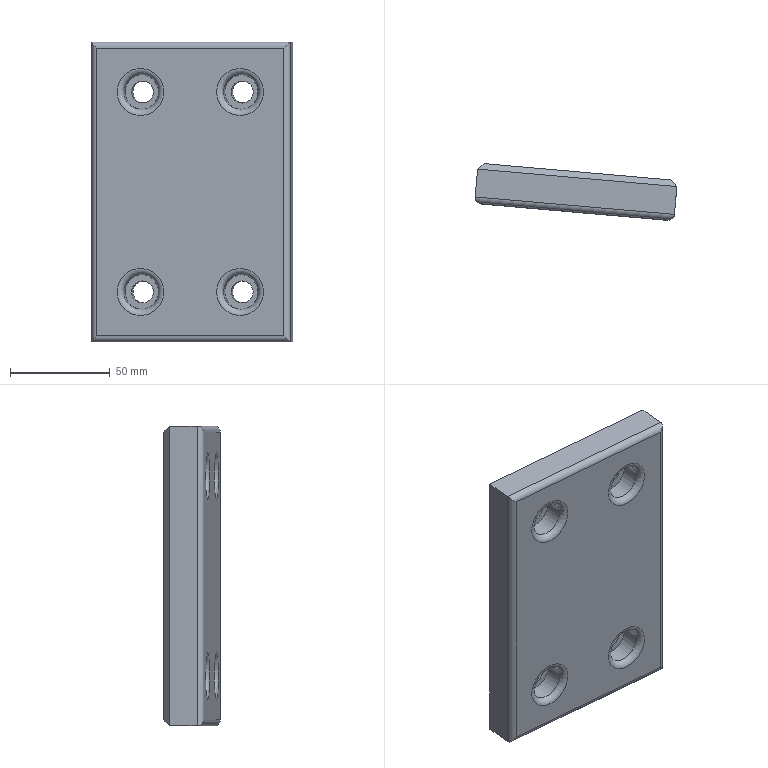Part | NX | features MAIN_BODY 2 | 1 solid | 30 faces | box 100.851 x 28.128 x 150 mm | volume 281787 mm3 | plane 14 | cylinder 12 | torus 4 | commonest cylinder face diameters 6 x4 11 x4 17.5 x4
STEP:
#1=CARTESIAN_POINT('',(223.712,-345.814,-117.));
#2=VERTEX_POINT('',#1);
#3=CARTESIAN_POINT('',(223.712,-345.814,27.));
#4=VERTEX_POINT('',#3);
#5=CARTESIAN_POINT('',(223.712,-345.814,30.));
#6=DIRECTION('',(0.,0.,-1.));
#7=VECTOR('',#6,1000.);
#8=LINE('',#5,#7);
#9=EDGE_CURVE('',#2,#4,#8,.F.);
#10=ORIENTED_EDGE('',*,*,#9,.F.);
#11=CARTESIAN_POINT('',(317.354,-354.006,-117.));
#12=VERTEX_POINT('',#11);
#13=CARTESIAN_POINT('',(190.837,-342.938,-117.));
#14=DIRECTION('',(0.9962,-0.08716,0.));
#15=VECTOR('',#14,1000.);
#16=LINE('',#13,#15);
#17=EDGE_CURVE('',#12,#2,#16,.F.);
#18=ORIENTED_EDGE('',*,*,#17,.F.);
#19=CARTESIAN_POINT('',(317.354,-354.006,27.));
#20=VERTEX_POINT('',#19);
#21=CARTESIAN_POINT('',(317.354,-354.006,-170.));
#22=DIRECTION('',(0.,0.,1.));
#23=VECTOR('',#22,1000.);
#24=LINE('',#21,#23);
#25=EDGE_CURVE('',#20,#12,#24,.F.);
#26=ORIENTED_EDGE('',*,*,#25,.F.);
#27=CARTESIAN_POINT('',(340.266,-356.011,27.));
#28=DIRECTION('',(-0.9962,0.08716,0.));
#29=VECTOR('',#28,1000.);
#30=LINE('',#27,#29);
#31=EDGE_CURVE('',#4,#20,#30,.F.);
#32=ORIENTED_EDGE('',*,*,#31,.F.);
#33=EDGE_LOOP('',(#10,#18,#26,#32));
#34=FACE_BOUND('',#33,.T.);
#35=CARTESIAN_POINT('',(245.628,-347.731,-6.75));
#36=VERTEX_POINT('',#35);
#37=CARTESIAN_POINT('',(245.628,-347.731,5.));
#38=DIRECTION('',(-0.08716,-0.9962,0.));
#39=DIRECTION('',(0.,0.,-1.));
#40=AXIS2_PLACEMENT_3D('',#37,#38,#39);
#41=CIRCLE('',#40,11.75);
#42=EDGE_CURVE('',#36,#36,#41,.T.);
#43=ORIENTED_EDGE('',*,*,#42,.F.);
#44=EDGE_LOOP('',(#43));
#45=FACE_BOUND('',#44,.T.);
#46=CARTESIAN_POINT('',(295.438,-352.089,-6.75));
#47=VERTEX_POINT('',#46);
#48=CARTESIAN_POINT('',(295.438,-352.089,5.));
#49=DIRECTION('',(-0.08716,-0.9962,0.));
#50=DIRECTION('',(0.,0.,-1.));
#51=AXIS2_PLACEMENT_3D('',#48,#49,#50);
#52=CIRCLE('',#51,11.75);
#53=EDGE_CURVE('',#47,#47,#52,.T.);
#54=ORIENTED_EDGE('',*,*,#53,.F.);
#55=EDGE_LOOP('',(#54));
#56=FACE_BOUND('',#55,.T.);
#57=CARTESIAN_POINT('',(295.438,-352.089,-106.75));
#58=VERTEX_POINT('',#57);
#59=CARTESIAN_POINT('',(295.438,-352.089,-95.));
#60=DIRECTION('',(-0.08716,-0.9962,0.));
#61=DIRECTION('',(0.,0.,-1.));
#62=AXIS2_PLACEMENT_3D('',#59,#60,#61);
#63=CIRCLE('',#62,11.75);
#64=EDGE_CURVE('',#58,#58,#63,.T.);
#65=ORIENTED_EDGE('',*,*,#64,.F.);
#66=EDGE_LOOP('',(#65));
#67=FACE_BOUND('',#66,.T.);
#68=CARTESIAN_POINT('',(245.628,-347.731,-106.75));
#69=VERTEX_POINT('',#68);
#70=CARTESIAN_POINT('',(245.628,-347.731,-95.));
#71=DIRECTION('',(-0.08716,-0.9962,0.));
#72=DIRECTION('',(0.,0.,-1.));
#73=AXIS2_PLACEMENT_3D('',#70,#71,#72);
#74=CIRCLE('',#73,11.75);
#75=EDGE_CURVE('',#69,#69,#74,.T.);
#76=ORIENTED_EDGE('',*,*,#75,.F.);
#77=EDGE_LOOP('',(#76));
#78=FACE_BOUND('',#77,.T.);
#79=CARTESIAN_POINT('',(190.837,-342.938,-170.));
#80=DIRECTION('',(0.08716,0.9962,0.));
#81=DIRECTION('',(0.,0.,-1.));
#82=AXIS2_PLACEMENT_3D('',#79,#80,#81);
#83=PLANE('',#82);
#84=ADVANCED_FACE('',(#34,#45,#56,#67,#78),#83,.F.);
#85=CARTESIAN_POINT('',(291.702,-331.686,-95.));
#86=VERTEX_POINT('',#85);
#87=CARTESIAN_POINT('',(297.181,-332.165,-95.));
#88=DIRECTION('',(0.08716,0.9962,0.));
#89=DIRECTION('',(-0.9962,0.08716,0.));
#90=AXIS2_PLACEMENT_3D('',#87,#88,#89);
#91=CIRCLE('',#90,5.5);
#92=EDGE_CURVE('',#86,#86,#91,.T.);
#93=ORIENTED_EDGE('',*,*,#92,.T.);
#94=EDGE_LOOP('',(#93));
#95=FACE_BOUND('',#94,.T.);
#96=CARTESIAN_POINT('',(296.484,-340.135,-89.5));
#97=VERTEX_POINT('',#96);
#98=CARTESIAN_POINT('',(296.484,-340.135,-95.));
#99=DIRECTION('',(0.08716,0.9962,0.));
#100=DIRECTION('',(0.,0.,1.));
#101=AXIS2_PLACEMENT_3D('',#98,#99,#100);
#102=CIRCLE('',#101,5.5);
#103=EDGE_CURVE('',#97,#97,#102,.T.);
#104=ORIENTED_EDGE('',*,*,#103,.F.);
#105=EDGE_LOOP('',(#104));
#106=FACE_BOUND('',#105,.T.);
#107=CARTESIAN_POINT('',(295.438,-352.089,-95.));
#108=DIRECTION('',(0.08716,0.9962,0.));
#109=DIRECTION('',(0.,0.,-1.));
#110=AXIS2_PLACEMENT_3D('',#107,#108,#109);
#111=CYLINDRICAL_SURFACE('',#110,5.5);
#112=ADVANCED_FACE('',(#95,#106),#111,.F.);
#113=CARTESIAN_POINT('',(252.85,-328.287,5.));
#114=VERTEX_POINT('',#113);
#115=CARTESIAN_POINT('',(247.371,-327.807,5.));
#116=DIRECTION('',(0.08716,0.9962,0.));
#117=DIRECTION('',(0.9962,-0.08716,0.));
#118=AXIS2_PLACEMENT_3D('',#115,#116,#117);
#119=CIRCLE('',#118,5.5);
#120=EDGE_CURVE('',#114,#114,#119,.T.);
#121=ORIENTED_EDGE('',*,*,#120,.T.);
#122=EDGE_LOOP('',(#121));
#123=FACE_BOUND('',#122,.T.);
#124=CARTESIAN_POINT('',(246.674,-335.777,10.5));
#125=VERTEX_POINT('',#124);
#126=CARTESIAN_POINT('',(246.674,-335.777,5.));
#127=DIRECTION('',(0.08716,0.9962,0.));
#128=DIRECTION('',(0.,0.,1.));
#129=AXIS2_PLACEMENT_3D('',#126,#127,#128);
#130=CIRCLE('',#129,5.5);
#131=EDGE_CURVE('',#125,#125,#130,.T.);
#132=ORIENTED_EDGE('',*,*,#131,.F.);
#133=EDGE_LOOP('',(#132));
#134=FACE_BOUND('',#133,.T.);
#135=CARTESIAN_POINT('',(245.628,-347.731,5.));
#136=DIRECTION('',(0.08716,0.9962,0.));
#137=DIRECTION('',(0.,0.,-1.));
#138=AXIS2_PLACEMENT_3D('',#135,#136,#137);
#139=CYLINDRICAL_SURFACE('',#138,5.5);
#140=ADVANCED_FACE('',(#123,#134),#139,.F.);
#141=CARTESIAN_POINT('',(319.097,-334.082,-117.));
#142=VERTEX_POINT('',#141);
#143=CARTESIAN_POINT('',(319.097,-334.082,27.));
#144=VERTEX_POINT('',#143);
#145=CARTESIAN_POINT('',(319.097,-334.082,-170.));
#146=DIRECTION('',(0.,0.,1.));
#147=VECTOR('',#146,1000.);
#148=LINE('',#145,#147);
#149=EDGE_CURVE('',#142,#144,#148,.T.);
#150=ORIENTED_EDGE('',*,*,#149,.F.);
#151=CARTESIAN_POINT('',(225.455,-325.89,-117.));
#152=VERTEX_POINT('',#151);
#153=CARTESIAN_POINT('',(192.58,-323.014,-117.));
#154=DIRECTION('',(0.9962,-0.08716,0.));
#155=VECTOR('',#154,1000.);
#156=LINE('',#153,#155);
#157=EDGE_CURVE('',#152,#142,#156,.T.);
#158=ORIENTED_EDGE('',*,*,#157,.F.);
#159=CARTESIAN_POINT('',(225.455,-325.89,27.));
#160=VERTEX_POINT('',#159);
#161=CARTESIAN_POINT('',(225.455,-325.89,-170.));
#162=DIRECTION('',(0.,0.,-1.));
#163=VECTOR('',#162,1000.);
#164=LINE('',#161,#163);
#165=EDGE_CURVE('',#160,#152,#164,.T.);
#166=ORIENTED_EDGE('',*,*,#165,.F.);
#167=CARTESIAN_POINT('',(192.58,-323.014,27.));
#168=DIRECTION('',(-0.9962,0.08716,0.));
#169=VECTOR('',#168,1000.);
#170=LINE('',#167,#169);
#171=EDGE_CURVE('',#144,#160,#170,.T.);
#172=ORIENTED_EDGE('',*,*,#171,.F.);
#173=EDGE_LOOP('',(#150,#158,#166,#172));
#174=FACE_BOUND('',#173,.T.);
#175=CARTESIAN_POINT('',(252.85,-328.287,-95.));
#176=VERTEX_POINT('',#175);
#177=CARTESIAN_POINT('',(247.371,-327.807,-95.));
#178=DIRECTION('',(-0.08716,-0.9962,0.));
#179=DIRECTION('',(0.9962,-0.08716,0.));
#180=AXIS2_PLACEMENT_3D('',#177,#178,#179);
#181=CIRCLE('',#180,5.5);
#182=EDGE_CURVE('',#176,#176,#181,.T.);
#183=ORIENTED_EDGE('',*,*,#182,.T.);
#184=EDGE_LOOP('',(#183));
#185=FACE_BOUND('',#184,.T.);
#186=ORIENTED_EDGE('',*,*,#92,.F.);
#187=EDGE_LOOP('',(#186));
#188=FACE_BOUND('',#187,.T.);
#189=CARTESIAN_POINT('',(291.702,-331.686,5.));
#190=VERTEX_POINT('',#189);
#191=CARTESIAN_POINT('',(297.181,-332.165,5.));
#192=DIRECTION('',(-0.08716,-0.9962,0.));
#193=DIRECTION('',(-0.9962,0.08716,0.));
#194=AXIS2_PLACEMENT_3D('',#191,#192,#193);
#195=CIRCLE('',#194,5.5);
#196=EDGE_CURVE('',#190,#190,#195,.T.);
#197=ORIENTED_EDGE('',*,*,#196,.T.);
#198=EDGE_LOOP('',(#197));
#199=FACE_BOUND('',#198,.T.);
#200=ORIENTED_EDGE('',*,*,#120,.F.);
#201=EDGE_LOOP('',(#200));
#202=FACE_BOUND('',#201,.T.);
#203=CARTESIAN_POINT('',(192.58,-323.014,-170.));
#204=DIRECTION('',(0.08716,0.9962,0.));
#205=DIRECTION('',(0.,0.,-1.));
#206=AXIS2_PLACEMENT_3D('',#203,#204,#205);
#207=PLANE('',#206);
#208=ADVANCED_FACE('',(#174,#185,#188,#199,#202),#207,.T.);
#209=CARTESIAN_POINT('',(220.985,-342.564,-120.));
#210=VERTEX_POINT('',#209);
#211=CARTESIAN_POINT('',(222.205,-328.617,-120.));
#212=VERTEX_POINT('',#211);
#213=CARTESIAN_POINT('',(220.723,-345.552,-120.));
#214=DIRECTION('',(0.08716,0.9962,0.));
#215=VECTOR('',#214,1000.);
#216=LINE('',#213,#215);
#217=EDGE_CURVE('',#210,#212,#216,.T.);
#218=ORIENTED_EDGE('',*,*,#217,.F.);
#219=CARTESIAN_POINT('',(220.985,-342.564,30.));
#220=VERTEX_POINT('',#219);
#221=CARTESIAN_POINT('',(220.985,-342.564,-170.));
#222=DIRECTION('',(0.,0.,-1.));
#223=VECTOR('',#222,1000.);
#224=LINE('',#221,#223);
#225=EDGE_CURVE('',#220,#210,#224,.T.);
#226=ORIENTED_EDGE('',*,*,#225,.F.);
#227=CARTESIAN_POINT('',(222.205,-328.617,30.));
#228=VERTEX_POINT('',#227);
#229=CARTESIAN_POINT('',(220.723,-345.552,30.));
#230=DIRECTION('',(0.08716,0.9962,0.));
#231=VECTOR('',#230,1000.);
#232=LINE('',#229,#231);
#233=EDGE_CURVE('',#220,#228,#232,.T.);
#234=ORIENTED_EDGE('',*,*,#233,.T.);
#235=CARTESIAN_POINT('',(222.205,-328.617,30.));
#236=DIRECTION('',(0.,0.,1.));
#237=VECTOR('',#236,1000.);
#238=LINE('',#235,#237);
#239=EDGE_CURVE('',#212,#228,#238,.T.);
#240=ORIENTED_EDGE('',*,*,#239,.F.);
#241=EDGE_LOOP('',(#218,#226,#234,#240));
#242=FACE_BOUND('',#241,.T.);
#243=CARTESIAN_POINT('',(220.723,-345.552,30.));
#244=DIRECTION('',(-0.9962,0.08716,0.));
#245=DIRECTION('',(0.,0.,1.));
#246=AXIS2_PLACEMENT_3D('',#243,#244,#245);
#247=PLANE('',#246);
#248=ADVANCED_FACE('',(#242),#247,.T.);
#249=CARTESIAN_POINT('',(320.604,-351.279,-120.));
#250=VERTEX_POINT('',#249);
#251=CARTESIAN_POINT('',(321.824,-337.332,-120.));
#252=VERTEX_POINT('',#251);
#253=CARTESIAN_POINT('',(320.343,-354.268,-120.));
#254=DIRECTION('',(0.08716,0.9962,0.));
#255=VECTOR('',#254,1000.);
#256=LINE('',#253,#255);
#257=EDGE_CURVE('',#250,#252,#256,.T.);
#258=ORIENTED_EDGE('',*,*,#257,.F.);
#259=CARTESIAN_POINT('',(340.528,-353.022,-120.));
#260=DIRECTION('',(0.9962,-0.08716,0.));
#261=VECTOR('',#260,1000.);
#262=LINE('',#259,#261);
#263=EDGE_CURVE('',#210,#250,#262,.T.);
#264=ORIENTED_EDGE('',*,*,#263,.F.);
#265=ORIENTED_EDGE('',*,*,#217,.T.);
#266=CARTESIAN_POINT('',(192.319,-326.002,-120.));
#267=DIRECTION('',(-0.9962,0.08716,0.));
#268=VECTOR('',#267,1000.);
#269=LINE('',#266,#268);
#270=EDGE_CURVE('',#252,#212,#269,.T.);
#271=ORIENTED_EDGE('',*,*,#270,.F.);
#272=EDGE_LOOP('',(#258,#264,#265,#271));
#273=FACE_BOUND('',#272,.T.);
#274=CARTESIAN_POINT('',(190.837,-342.938,-120.));
#275=DIRECTION('',(0.,0.,-1.));
#276=DIRECTION('',(-0.9962,0.08716,0.));
#277=AXIS2_PLACEMENT_3D('',#274,#275,#276);
#278=PLANE('',#277);
#279=ADVANCED_FACE('',(#273),#278,.T.);
#280=CARTESIAN_POINT('',(320.604,-351.279,30.));
#281=VERTEX_POINT('',#280);
#282=CARTESIAN_POINT('',(321.824,-337.332,30.));
#283=VERTEX_POINT('',#282);
#284=CARTESIAN_POINT('',(320.343,-354.268,30.));
#285=DIRECTION('',(0.08716,0.9962,0.));
#286=VECTOR('',#285,1000.);
#287=LINE('',#284,#286);
#288=EDGE_CURVE('',#281,#283,#287,.T.);
#289=ORIENTED_EDGE('',*,*,#288,.F.);
#290=CARTESIAN_POINT('',(320.604,-351.279,30.));
#291=DIRECTION('',(0.,0.,1.));
#292=VECTOR('',#291,1000.);
#293=LINE('',#290,#292);
#294=EDGE_CURVE('',#250,#281,#293,.T.);
#295=ORIENTED_EDGE('',*,*,#294,.F.);
#296=ORIENTED_EDGE('',*,*,#257,.T.);
#297=CARTESIAN_POINT('',(321.824,-337.332,-170.));
#298=DIRECTION('',(0.,0.,-1.));
#299=VECTOR('',#298,1000.);
#300=LINE('',#297,#299);
#301=EDGE_CURVE('',#283,#252,#300,.T.);
#302=ORIENTED_EDGE('',*,*,#301,.F.);
#303=EDGE_LOOP('',(#289,#295,#296,#302));
#304=FACE_BOUND('',#303,.T.);
#305=CARTESIAN_POINT('',(320.343,-354.268,-170.));
#306=DIRECTION('',(0.9962,-0.08716,0.));
#307=DIRECTION('',(0.,0.,-1.));
#308=AXIS2_PLACEMENT_3D('',#305,#306,#307);
#309=PLANE('',#308);
#310=ADVANCED_FACE('',(#304),#309,.T.);
#311=ORIENTED_EDGE('',*,*,#233,.F.);
#312=CARTESIAN_POINT('',(191.099,-339.949,30.));
#313=DIRECTION('',(-0.9962,0.08716,0.));
#314=VECTOR('',#313,1000.);
#315=LINE('',#312,#314);
#316=EDGE_CURVE('',#281,#220,#315,.T.);
#317=ORIENTED_EDGE('',*,*,#316,.F.);
#318=ORIENTED_EDGE('',*,*,#288,.T.);
#319=CARTESIAN_POINT('',(341.748,-339.076,30.));
#320=DIRECTION('',(0.9962,-0.08716,0.));
#321=VECTOR('',#320,1000.);
#322=LINE('',#319,#321);
#323=EDGE_CURVE('',#228,#283,#322,.T.);
#324=ORIENTED_EDGE('',*,*,#323,.F.);
#325=EDGE_LOOP('',(#311,#317,#318,#324));
#326=FACE_BOUND('',#325,.T.);
#327=CARTESIAN_POINT('',(340.266,-356.011,30.));
#328=DIRECTION('',(0.,0.,1.));
#329=DIRECTION('',(0.9962,-0.08716,0.));
#330=AXIS2_PLACEMENT_3D('',#327,#328,#329);
#331=PLANE('',#330);
#332=ADVANCED_FACE('',(#326),#331,.T.);
#333=CARTESIAN_POINT('',(296.484,-340.135,-0.5));
#334=VERTEX_POINT('',#333);
#335=CARTESIAN_POINT('',(296.484,-340.135,5.));
#336=DIRECTION('',(-0.08716,-0.9962,0.));
#337=DIRECTION('',(0.,0.,-1.));
#338=AXIS2_PLACEMENT_3D('',#335,#336,#337);
#339=CIRCLE('',#338,5.5);
#340=EDGE_CURVE('',#334,#334,#339,.F.);
#341=ORIENTED_EDGE('',*,*,#340,.F.);
#342=EDGE_LOOP('',(#341));
#343=FACE_BOUND('',#342,.T.);
#344=ORIENTED_EDGE('',*,*,#196,.F.);
#345=EDGE_LOOP('',(#344));
#346=FACE_BOUND('',#345,.T.);
#347=CARTESIAN_POINT('',(295.438,-352.089,5.));
#348=DIRECTION('',(0.08716,0.9962,0.));
#349=DIRECTION('',(0.,0.,-1.));
#350=AXIS2_PLACEMENT_3D('',#347,#348,#349);
#351=CYLINDRICAL_SURFACE('',#350,5.5);
#352=ADVANCED_FACE('',(#343,#346),#351,.F.);
#353=CARTESIAN_POINT('',(246.674,-335.777,-100.5));
#354=VERTEX_POINT('',#353);
#355=CARTESIAN_POINT('',(246.674,-335.777,-95.));
#356=DIRECTION('',(-0.08716,-0.9962,0.));
#357=DIRECTION('',(0.,0.,-1.));
#358=AXIS2_PLACEMENT_3D('',#355,#356,#357);
#359=CIRCLE('',#358,5.5);
#360=EDGE_CURVE('',#354,#354,#359,.F.);
#361=ORIENTED_EDGE('',*,*,#360,.F.);
#362=EDGE_LOOP('',(#361));
#363=FACE_BOUND('',#362,.T.);
#364=ORIENTED_EDGE('',*,*,#182,.F.);
#365=EDGE_LOOP('',(#364));
#366=FACE_BOUND('',#365,.T.);
#367=CARTESIAN_POINT('',(245.628,-347.731,-95.));
#368=DIRECTION('',(0.08716,0.9962,0.));
#369=DIRECTION('',(0.,0.,-1.));
#370=AXIS2_PLACEMENT_3D('',#367,#368,#369);
#371=CYLINDRICAL_SURFACE('',#370,5.5);
#372=ADVANCED_FACE('',(#363,#366),#371,.F.);
#373=CARTESIAN_POINT('',(245.889,-344.743,-3.75));
#374=VERTEX_POINT('',#373);
#375=CARTESIAN_POINT('',(245.889,-344.743,5.));
#376=DIRECTION('',(-0.08716,-0.9962,0.));
#377=DIRECTION('',(0.,0.,-1.));
#378=AXIS2_PLACEMENT_3D('',#375,#376,#377);
#379=CIRCLE('',#378,8.75);
#380=EDGE_CURVE('',#374,#374,#379,.F.);
#381=ORIENTED_EDGE('',*,*,#380,.F.);
#382=EDGE_LOOP('',(#381));
#383=FACE_BOUND('',#382,.T.);
#384=CARTESIAN_POINT('',(255.39,-336.539,5.));
#385=VERTEX_POINT('',#384);
#386=CARTESIAN_POINT('',(246.674,-335.777,5.));
#387=DIRECTION('',(0.08716,0.9962,0.));
#388=DIRECTION('',(0.9962,-0.08716,0.));
#389=AXIS2_PLACEMENT_3D('',#386,#387,#388);
#390=CIRCLE('',#389,8.75);
#391=EDGE_CURVE('',#385,#385,#390,.T.);
#392=ORIENTED_EDGE('',*,*,#391,.T.);
#393=EDGE_LOOP('',(#392));
#394=FACE_BOUND('',#393,.T.);
#395=CARTESIAN_POINT('',(244.756,-357.693,5.));
#396=DIRECTION('',(0.08716,0.9962,0.));
#397=DIRECTION('',(0.,0.,-1.));
#398=AXIS2_PLACEMENT_3D('',#395,#396,#397);
#399=CYLINDRICAL_SURFACE('',#398,8.75);
#400=ADVANCED_FACE('',(#383,#394),#399,.F.);
#401=ORIENTED_EDGE('',*,*,#131,.T.);
#402=EDGE_LOOP('',(#401));
#403=FACE_BOUND('',#402,.T.);
#404=ORIENTED_EDGE('',*,*,#391,.F.);
#405=EDGE_LOOP('',(#404));
#406=FACE_BOUND('',#405,.T.);
#407=CARTESIAN_POINT('',(246.674,-335.777,5.));
#408=DIRECTION('',(-0.08716,-0.9962,0.));
#409=DIRECTION('',(0.,0.,1.));
#410=AXIS2_PLACEMENT_3D('',#407,#408,#409);
#411=PLANE('',#410);
#412=ADVANCED_FACE('',(#403,#406),#411,.T.);
#413=CARTESIAN_POINT('',(245.889,-344.743,-103.75));
#414=VERTEX_POINT('',#413);
#415=CARTESIAN_POINT('',(245.889,-344.743,-95.));
#416=DIRECTION('',(-0.08716,-0.9962,0.));
#417=DIRECTION('',(0.,0.,-1.));
#418=AXIS2_PLACEMENT_3D('',#415,#416,#417);
#419=CIRCLE('',#418,8.75);
#420=EDGE_CURVE('',#414,#414,#419,.F.);
#421=ORIENTED_EDGE('',*,*,#420,.F.);
#422=EDGE_LOOP('',(#421));
#423=FACE_BOUND('',#422,.T.);
#424=CARTESIAN_POINT('',(255.39,-336.539,-95.));
#425=VERTEX_POINT('',#424);
#426=CARTESIAN_POINT('',(246.674,-335.777,-95.));
#427=DIRECTION('',(-0.08716,-0.9962,0.));
#428=DIRECTION('',(0.9962,-0.08716,0.));
#429=AXIS2_PLACEMENT_3D('',#426,#427,#428);
#430=CIRCLE('',#429,8.75);
#431=EDGE_CURVE('',#425,#425,#430,.T.);
#432=ORIENTED_EDGE('',*,*,#431,.F.);
#433=EDGE_LOOP('',(#432));
#434=FACE_BOUND('',#433,.T.);
#435=CARTESIAN_POINT('',(244.756,-357.693,-95.));
#436=DIRECTION('',(0.08716,0.9962,0.));
#437=DIRECTION('',(0.,0.,-1.));
#438=AXIS2_PLACEMENT_3D('',#435,#436,#437);
#439=CYLINDRICAL_SURFACE('',#438,8.75);
#440=ADVANCED_FACE('',(#423,#434),#439,.F.);
#441=ORIENTED_EDGE('',*,*,#431,.T.);
#442=EDGE_LOOP('',(#441));
#443=FACE_BOUND('',#442,.T.);
#444=ORIENTED_EDGE('',*,*,#360,.T.);
#445=EDGE_LOOP('',(#444));
#446=FACE_BOUND('',#445,.T.);
#447=CARTESIAN_POINT('',(246.674,-335.777,-95.));
#448=DIRECTION('',(0.08716,0.9962,0.));
#449=DIRECTION('',(0.,0.,-1.));
#450=AXIS2_PLACEMENT_3D('',#447,#448,#449);
#451=PLANE('',#450);
#452=ADVANCED_FACE('',(#443,#446),#451,.F.);
#453=CARTESIAN_POINT('',(295.699,-349.1,-3.75));
#454=VERTEX_POINT('',#453);
#455=CARTESIAN_POINT('',(295.699,-349.1,5.));
#456=DIRECTION('',(-0.08716,-0.9962,0.));
#457=DIRECTION('',(0.,0.,-1.));
#458=AXIS2_PLACEMENT_3D('',#455,#456,#457);
#459=CIRCLE('',#458,8.75);
#460=EDGE_CURVE('',#454,#454,#459,.F.);
#461=ORIENTED_EDGE('',*,*,#460,.F.);
#462=EDGE_LOOP('',(#461));
#463=FACE_BOUND('',#462,.T.);
#464=CARTESIAN_POINT('',(287.767,-339.372,5.));
#465=VERTEX_POINT('',#464);
#466=CARTESIAN_POINT('',(296.484,-340.135,5.));
#467=DIRECTION('',(-0.08716,-0.9962,0.));
#468=DIRECTION('',(-0.9962,0.08716,0.));
#469=AXIS2_PLACEMENT_3D('',#466,#467,#468);
#470=CIRCLE('',#469,8.75);
#471=EDGE_CURVE('',#465,#465,#470,.T.);
#472=ORIENTED_EDGE('',*,*,#471,.F.);
#473=EDGE_LOOP('',(#472));
#474=FACE_BOUND('',#473,.T.);
#475=CARTESIAN_POINT('',(294.566,-362.051,5.));
#476=DIRECTION('',(0.08716,0.9962,0.));
#477=DIRECTION('',(0.,0.,-1.));
#478=AXIS2_PLACEMENT_3D('',#475,#476,#477);
#479=CYLINDRICAL_SURFACE('',#478,8.75);
#480=ADVANCED_FACE('',(#463,#474),#479,.F.);
#481=ORIENTED_EDGE('',*,*,#471,.T.);
#482=EDGE_LOOP('',(#481));
#483=FACE_BOUND('',#482,.T.);
#484=ORIENTED_EDGE('',*,*,#340,.T.);
#485=EDGE_LOOP('',(#484));
#486=FACE_BOUND('',#485,.T.);
#487=CARTESIAN_POINT('',(296.484,-340.135,5.));
#488=DIRECTION('',(0.08716,0.9962,0.));
#489=DIRECTION('',(0.,0.,-1.));
#490=AXIS2_PLACEMENT_3D('',#487,#488,#489);
#491=PLANE('',#490);
#492=ADVANCED_FACE('',(#483,#486),#491,.F.);
#493=CARTESIAN_POINT('',(295.699,-349.1,-103.75));
#494=VERTEX_POINT('',#493);
#495=CARTESIAN_POINT('',(295.699,-349.1,-95.));
#496=DIRECTION('',(-0.08716,-0.9962,0.));
#497=DIRECTION('',(0.,0.,-1.));
#498=AXIS2_PLACEMENT_3D('',#495,#496,#497);
#499=CIRCLE('',#498,8.75);
#500=EDGE_CURVE('',#494,#494,#499,.F.);
#501=ORIENTED_EDGE('',*,*,#500,.F.);
#502=EDGE_LOOP('',(#501));
#503=FACE_BOUND('',#502,.T.);
#504=CARTESIAN_POINT('',(287.767,-339.372,-95.));
#505=VERTEX_POINT('',#504);
#506=CARTESIAN_POINT('',(296.484,-340.135,-95.));
#507=DIRECTION('',(0.08716,0.9962,0.));
#508=DIRECTION('',(-0.9962,0.08716,0.));
#509=AXIS2_PLACEMENT_3D('',#506,#507,#508);
#510=CIRCLE('',#509,8.75);
#511=EDGE_CURVE('',#505,#505,#510,.T.);
#512=ORIENTED_EDGE('',*,*,#511,.T.);
#513=EDGE_LOOP('',(#512));
#514=FACE_BOUND('',#513,.T.);
#515=CARTESIAN_POINT('',(294.566,-362.051,-95.));
#516=DIRECTION('',(0.08716,0.9962,0.));
#517=DIRECTION('',(0.,0.,-1.));
#518=AXIS2_PLACEMENT_3D('',#515,#516,#517);
#519=CYLINDRICAL_SURFACE('',#518,8.75);
#520=ADVANCED_FACE('',(#503,#514),#519,.F.);
#521=ORIENTED_EDGE('',*,*,#103,.T.);
#522=EDGE_LOOP('',(#521));
#523=FACE_BOUND('',#522,.T.);
#524=ORIENTED_EDGE('',*,*,#511,.F.);
#525=EDGE_LOOP('',(#524));
#526=FACE_BOUND('',#525,.T.);
#527=CARTESIAN_POINT('',(296.484,-340.135,-95.));
#528=DIRECTION('',(-0.08716,-0.9962,0.));
#529=DIRECTION('',(0.,0.,1.));
#530=AXIS2_PLACEMENT_3D('',#527,#528,#529);
#531=PLANE('',#530);
#532=ADVANCED_FACE('',(#523,#526),#531,.T.);
#533=CARTESIAN_POINT('',(223.973,-342.825,-117.));
#534=DIRECTION('',(0.7044,-0.06163,-0.7071));
#535=DIRECTION('',(-0.7044,0.06163,-0.7071));
#536=AXIS2_PLACEMENT_3D('',#533,#534,#535);
#537=ELLIPSE('',#536,4.243,3.);
#538=EDGE_CURVE('',#2,#210,#537,.T.);
#539=ORIENTED_EDGE('',*,*,#538,.T.);
#540=ORIENTED_EDGE('',*,*,#263,.T.);
#541=CARTESIAN_POINT('',(317.615,-351.018,-117.));
#542=DIRECTION('',(0.7044,-0.06163,0.7071));
#543=DIRECTION('',(-0.7044,0.06163,0.7071));
#544=AXIS2_PLACEMENT_3D('',#541,#542,#543);
#545=ELLIPSE('',#544,4.243,3.);
#546=EDGE_CURVE('',#250,#12,#545,.F.);
#547=ORIENTED_EDGE('',*,*,#546,.T.);
#548=ORIENTED_EDGE('',*,*,#17,.T.);
#549=EDGE_LOOP('',(#539,#540,#547,#548));
#550=FACE_BOUND('',#549,.T.);
#551=CARTESIAN_POINT('',(191.099,-339.949,-117.));
#552=DIRECTION('',(-0.9962,0.08716,0.));
#553=DIRECTION('',(0.,0.,1.));
#554=AXIS2_PLACEMENT_3D('',#551,#552,#553);
#555=CYLINDRICAL_SURFACE('',#554,3.);
#556=ADVANCED_FACE('',(#550),#555,.T.);
#557=ORIENTED_EDGE('',*,*,#546,.F.);
#558=ORIENTED_EDGE('',*,*,#294,.T.);
#559=CARTESIAN_POINT('',(317.615,-351.018,27.));
#560=DIRECTION('',(-0.7044,0.06163,0.7071));
#561=DIRECTION('',(-0.7044,0.06163,-0.7071));
#562=AXIS2_PLACEMENT_3D('',#559,#560,#561);
#563=ELLIPSE('',#562,4.243,3.);
#564=EDGE_CURVE('',#281,#20,#563,.F.);
#565=ORIENTED_EDGE('',*,*,#564,.T.);
#566=ORIENTED_EDGE('',*,*,#25,.T.);
#567=EDGE_LOOP('',(#557,#558,#565,#566));
#568=FACE_BOUND('',#567,.T.);
#569=CARTESIAN_POINT('',(317.615,-351.018,-170.));
#570=DIRECTION('',(0.,0.,-1.));
#571=DIRECTION('',(-0.08716,-0.9962,0.));
#572=AXIS2_PLACEMENT_3D('',#569,#570,#571);
#573=CYLINDRICAL_SURFACE('',#572,3.);
#574=ADVANCED_FACE('',(#568),#573,.T.);
#575=ORIENTED_EDGE('',*,*,#538,.F.);
#576=ORIENTED_EDGE('',*,*,#9,.T.);
#577=CARTESIAN_POINT('',(223.973,-342.825,27.));
#578=DIRECTION('',(-0.7044,0.06163,-0.7071));
#579=DIRECTION('',(-0.7044,0.06163,0.7071));
#580=AXIS2_PLACEMENT_3D('',#577,#578,#579);
#581=ELLIPSE('',#580,4.243,3.);
#582=EDGE_CURVE('',#4,#220,#581,.T.);
#583=ORIENTED_EDGE('',*,*,#582,.T.);
#584=ORIENTED_EDGE('',*,*,#225,.T.);
#585=EDGE_LOOP('',(#575,#576,#583,#584));
#586=FACE_BOUND('',#585,.T.);
#587=CARTESIAN_POINT('',(223.973,-342.825,30.));
#588=DIRECTION('',(0.,0.,1.));
#589=DIRECTION('',(0.9962,-0.08716,0.));
#590=AXIS2_PLACEMENT_3D('',#587,#588,#589);
#591=CYLINDRICAL_SURFACE('',#590,3.);
#592=ADVANCED_FACE('',(#586),#591,.T.);
#593=ORIENTED_EDGE('',*,*,#564,.F.);
#594=ORIENTED_EDGE('',*,*,#316,.T.);
#595=ORIENTED_EDGE('',*,*,#582,.F.);
#596=ORIENTED_EDGE('',*,*,#31,.T.);
#597=EDGE_LOOP('',(#593,#594,#595,#596));
#598=FACE_BOUND('',#597,.T.);
#599=CARTESIAN_POINT('',(340.528,-353.022,27.));
#600=DIRECTION('',(0.9962,-0.08716,0.));
#601=DIRECTION('',(0.,0.,-1.));
#602=AXIS2_PLACEMENT_3D('',#599,#600,#601);
#603=CYLINDRICAL_SURFACE('',#602,3.);
#604=ADVANCED_FACE('',(#598),#603,.T.);
#605=ORIENTED_EDGE('',*,*,#42,.T.);
#606=EDGE_LOOP('',(#605));
#607=FACE_BOUND('',#606,.T.);
#608=ORIENTED_EDGE('',*,*,#380,.T.);
#609=EDGE_LOOP('',(#608));
#610=FACE_BOUND('',#609,.T.);
#611=CARTESIAN_POINT('',(245.889,-344.743,5.));
#612=DIRECTION('',(0.08716,0.9962,0.));
#613=DIRECTION('',(0.,0.,-1.));
#614=AXIS2_PLACEMENT_3D('',#611,#612,#613);
#615=TOROIDAL_SURFACE('',#614,11.75,3.);
#616=ADVANCED_FACE('',(#607,#610),#615,.T.);
#617=ORIENTED_EDGE('',*,*,#460,.T.);
#618=EDGE_LOOP('',(#617));
#619=FACE_BOUND('',#618,.T.);
#620=ORIENTED_EDGE('',*,*,#53,.T.);
#621=EDGE_LOOP('',(#620));
#622=FACE_BOUND('',#621,.T.);
#623=CARTESIAN_POINT('',(295.699,-349.1,5.));
#624=DIRECTION('',(0.08716,0.9962,0.));
#625=DIRECTION('',(0.,0.,-1.));
#626=AXIS2_PLACEMENT_3D('',#623,#624,#625);
#627=TOROIDAL_SURFACE('',#626,11.75,3.);
#628=ADVANCED_FACE('',(#619,#622),#627,.T.);
#629=ORIENTED_EDGE('',*,*,#64,.T.);
#630=EDGE_LOOP('',(#629));
#631=FACE_BOUND('',#630,.T.);
#632=ORIENTED_EDGE('',*,*,#500,.T.);
#633=EDGE_LOOP('',(#632));
#634=FACE_BOUND('',#633,.T.);
#635=CARTESIAN_POINT('',(295.699,-349.1,-95.));
#636=DIRECTION('',(0.08716,0.9962,0.));
#637=DIRECTION('',(0.,0.,-1.));
#638=AXIS2_PLACEMENT_3D('',#635,#636,#637);
#639=TOROIDAL_SURFACE('',#638,11.75,3.);
#640=ADVANCED_FACE('',(#631,#634),#639,.T.);
#641=ORIENTED_EDGE('',*,*,#420,.T.);
#642=EDGE_LOOP('',(#641));
#643=FACE_BOUND('',#642,.T.);
#644=ORIENTED_EDGE('',*,*,#75,.T.);
#645=EDGE_LOOP('',(#644));
#646=FACE_BOUND('',#645,.T.);
#647=CARTESIAN_POINT('',(245.889,-344.743,-95.));
#648=DIRECTION('',(0.08716,0.9962,0.));
#649=DIRECTION('',(0.,0.,-1.));
#650=AXIS2_PLACEMENT_3D('',#647,#648,#649);
#651=TOROIDAL_SURFACE('',#650,11.75,3.);
#652=ADVANCED_FACE('',(#643,#646),#651,.T.);
#653=CARTESIAN_POINT('',(224.371,-326.799,-118.));
#654=DIRECTION('',(-0.6255,-0.5248,-0.5774));
#655=VECTOR('',#654,1000.);
#656=LINE('',#653,#655);
#657=EDGE_CURVE('',#212,#152,#656,.F.);
#658=ORIENTED_EDGE('',*,*,#657,.T.);
#659=ORIENTED_EDGE('',*,*,#157,.T.);
#660=CARTESIAN_POINT('',(320.006,-335.166,-118.));
#661=DIRECTION('',(0.5248,-0.6255,-0.5774));
#662=VECTOR('',#661,1000.);
#663=LINE('',#660,#662);
#664=EDGE_CURVE('',#142,#252,#663,.T.);
#665=ORIENTED_EDGE('',*,*,#664,.T.);
#666=ORIENTED_EDGE('',*,*,#270,.T.);
#667=EDGE_LOOP('',(#658,#659,#665,#666));
#668=FACE_BOUND('',#667,.T.);
#669=CARTESIAN_POINT('',(192.58,-323.014,-117.));
#670=DIRECTION('',(-0.06163,-0.7044,0.7071));
#671=DIRECTION('',(0.06163,0.7044,0.7071));
#672=AXIS2_PLACEMENT_3D('',#669,#670,#671);
#673=PLANE('',#672);
#674=ADVANCED_FACE('',(#668),#673,.F.);
#675=ORIENTED_EDGE('',*,*,#664,.F.);
#676=ORIENTED_EDGE('',*,*,#149,.T.);
#677=CARTESIAN_POINT('',(259.404,-262.942,-38.667));
#678=DIRECTION('',(-0.5248,0.6255,-0.5774));
#679=VECTOR('',#678,1000.);
#680=LINE('',#677,#679);
#681=EDGE_CURVE('',#144,#283,#680,.F.);
#682=ORIENTED_EDGE('',*,*,#681,.T.);
#683=ORIENTED_EDGE('',*,*,#301,.T.);
#684=EDGE_LOOP('',(#675,#676,#682,#683));
#685=FACE_BOUND('',#684,.T.);
#686=CARTESIAN_POINT('',(319.097,-334.082,-170.));
#687=DIRECTION('',(-0.766,-0.6428,0.));
#688=DIRECTION('',(0.6428,-0.766,0.));
#689=AXIS2_PLACEMENT_3D('',#686,#687,#688);
#690=PLANE('',#689);
#691=ADVANCED_FACE('',(#685),#690,.F.);
#692=ORIENTED_EDGE('',*,*,#657,.F.);
#693=ORIENTED_EDGE('',*,*,#239,.T.);
#694=CARTESIAN_POINT('',(296.595,-266.196,-38.667));
#695=DIRECTION('',(-0.6255,-0.5248,0.5774));
#696=VECTOR('',#695,1000.);
#697=LINE('',#694,#696);
#698=EDGE_CURVE('',#228,#160,#697,.F.);
#699=ORIENTED_EDGE('',*,*,#698,.T.);
#700=ORIENTED_EDGE('',*,*,#165,.T.);
#701=EDGE_LOOP('',(#692,#693,#699,#700));
#702=FACE_BOUND('',#701,.T.);
#703=CARTESIAN_POINT('',(225.455,-325.89,-170.));
#704=DIRECTION('',(0.6428,-0.766,0.));
#705=DIRECTION('',(0.766,0.6428,0.));
#706=AXIS2_PLACEMENT_3D('',#703,#704,#705);
#707=PLANE('',#706);
#708=ADVANCED_FACE('',(#702),#707,.F.);
#709=ORIENTED_EDGE('',*,*,#681,.F.);
#710=ORIENTED_EDGE('',*,*,#171,.T.);
#711=ORIENTED_EDGE('',*,*,#698,.F.);
#712=ORIENTED_EDGE('',*,*,#323,.T.);
#713=EDGE_LOOP('',(#709,#710,#711,#712));
#714=FACE_BOUND('',#713,.T.);
#715=CARTESIAN_POINT('',(192.58,-323.014,27.));
#716=DIRECTION('',(-0.06163,-0.7044,-0.7071));
#717=DIRECTION('',(-0.06163,-0.7044,0.7071));
#718=AXIS2_PLACEMENT_3D('',#715,#716,#717);
#719=PLANE('',#718);
#720=ADVANCED_FACE('',(#714),#719,.F.);
#721=CLOSED_SHELL('',(#84,#112,#140,#208,#248,#279,#310,#332,#352,#372,#400,#412,#440,#452,#480,#492,#520,#532,#556,#574,#592,#604,#616,#628,#640,#652,#674,#691,#708,#720));
#722=MANIFOLD_SOLID_BREP('',#721);
#723=(LENGTH_UNIT()NAMED_UNIT(*)SI_UNIT(.MILLI.,.METRE.));
#724=UNCERTAINTY_MEASURE_WITH_UNIT(LENGTH_MEASURE(0.00001),#723,'','');
#725=(NAMED_UNIT(*)PLANE_ANGLE_UNIT()SI_UNIT($,.RADIAN.));
#726=(NAMED_UNIT(*)SI_UNIT($,.STERADIAN.)SOLID_ANGLE_UNIT());
#727=(GEOMETRIC_REPRESENTATION_CONTEXT(3)GLOBAL_UNCERTAINTY_ASSIGNED_CONTEXT((#724))GLOBAL_UNIT_ASSIGNED_CONTEXT((#723,#725,#726))REPRESENTATION_CONTEXT('',''));
#728=ADVANCED_BREP_SHAPE_REPRESENTATION('',(#722),#727);